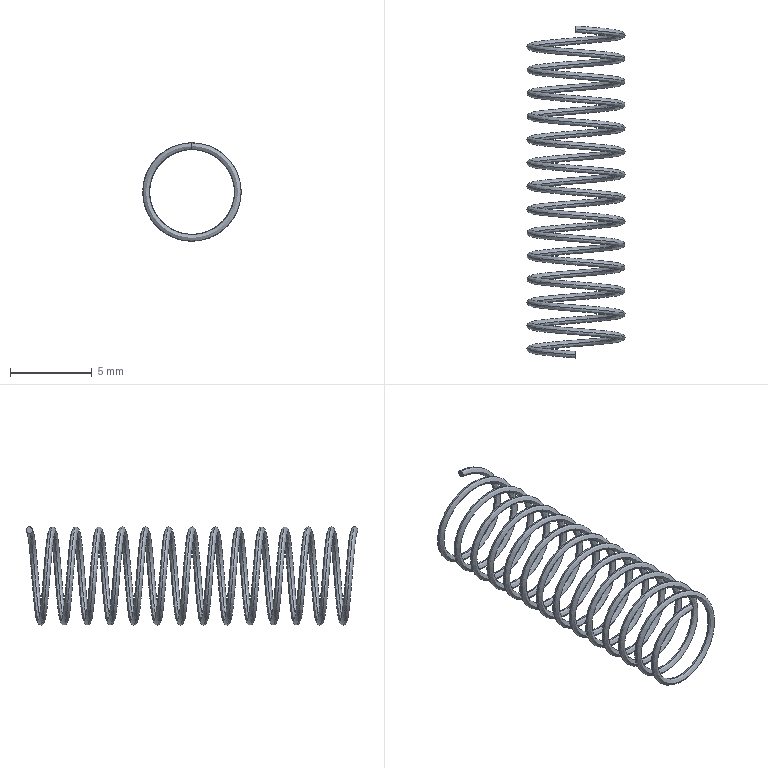Part | SolidWorks | features Helix 1, RefAxis 1, Sweep 1 | 1 solid | 4 faces | box 6 x 20.28 x 6 mm | volume 31.046 mm3 | spline 2 | plane 2